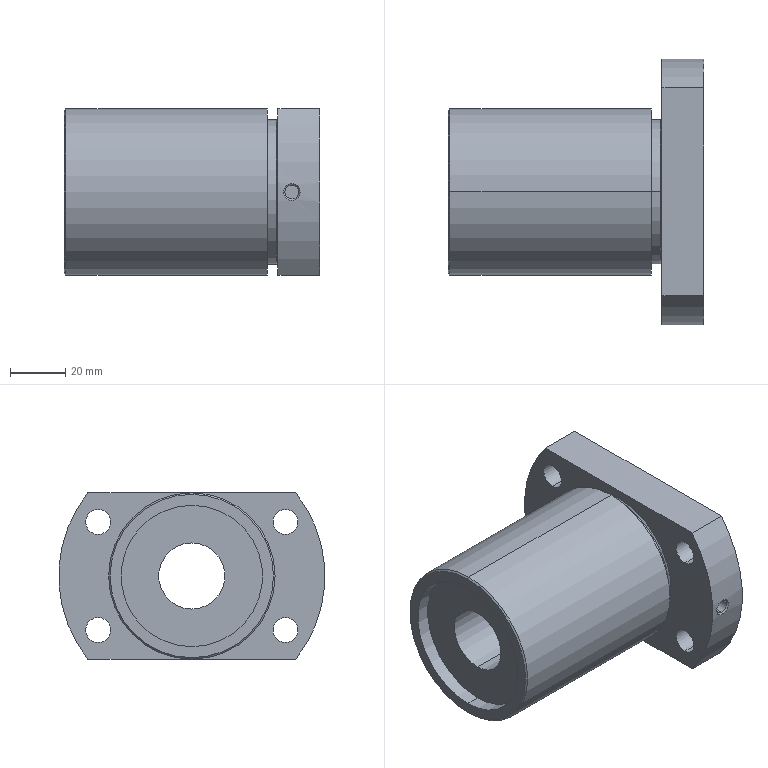Part | STEP file | 0244_Z_001_BSST2510-1195_2 | 1 solid | 39 faces | box 92 x 96 x 60 mm | volume 221226 mm3 | cylinder 24 | plane 9 | cone 4 | spline 2 | commonest cylinder face diameters 9 x8 51 x4 5 x2 23.855 x2 47 x2 52.3 x2